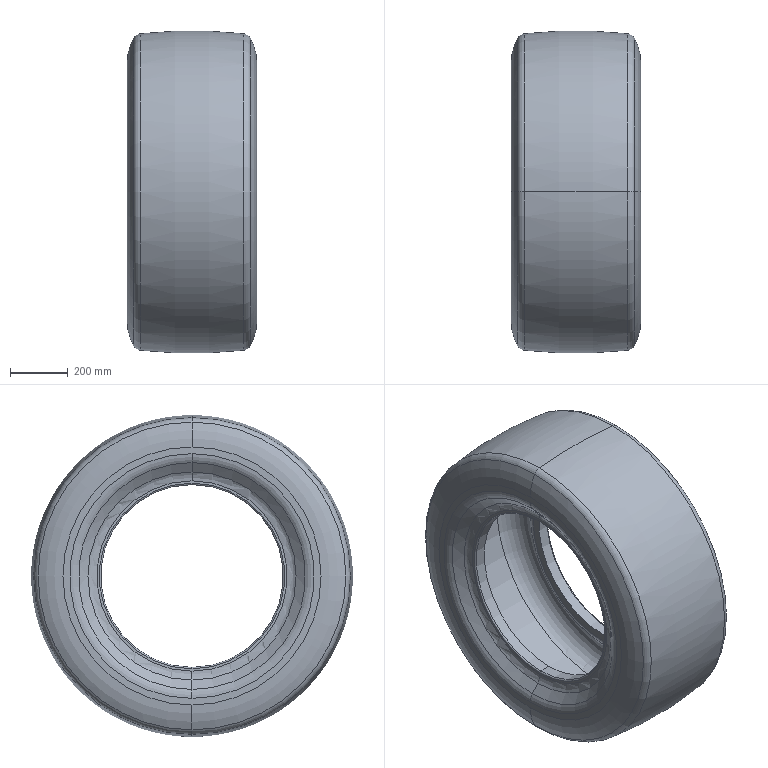Part | SolidWorks | features RevCut 1, Revolution 1 | 1 solid | 50 faces | box 450 x 1120 x 1120 mm | volume 112595756 mm3 | torus 30 | cone 8 | plane 6 | cylinder 6 | commonest cylinder face diameters 635 x4 1016 x2
STEP:
#1=CARTESIAN_POINT('',(142.639,0.,365.878));
#2=VERTEX_POINT('',#1);
#3=CARTESIAN_POINT('',(142.639,0.,-365.878));
#4=VERTEX_POINT('',#3);
#5=CARTESIAN_POINT('',(142.639,0.,0.));
#6=DIRECTION('',(-1.,0.,0.));
#7=DIRECTION('',(0.,0.,1.));
#8=AXIS2_PLACEMENT_3D('',#5,#6,#7);
#9=CIRCLE('',#8,365.878);
#10=EDGE_CURVE('',#2,#4,#9,.T.);
#11=ORIENTED_EDGE('',*,*,#10,.T.);
#12=CARTESIAN_POINT('',(134.,0.,-344.814));
#13=VERTEX_POINT('',#12);
#14=CARTESIAN_POINT('',(164.,0.,-344.814));
#15=DIRECTION('',(0.,1.,0.));
#16=DIRECTION('',(0.,0.,1.));
#17=AXIS2_PLACEMENT_3D('',#14,#15,#16);
#18=CIRCLE('',#17,30.);
#19=EDGE_CURVE('',#4,#13,#18,.T.);
#20=ORIENTED_EDGE('',*,*,#19,.T.);
#21=CARTESIAN_POINT('',(134.,0.,344.814));
#22=VERTEX_POINT('',#21);
#23=CARTESIAN_POINT('',(134.,0.,0.));
#24=DIRECTION('',(-1.,0.,0.));
#25=DIRECTION('',(0.,0.,1.));
#26=AXIS2_PLACEMENT_3D('',#23,#24,#25);
#27=CIRCLE('',#26,344.814);
#28=EDGE_CURVE('',#22,#13,#27,.T.);
#29=ORIENTED_EDGE('',*,*,#28,.F.);
#30=CARTESIAN_POINT('',(164.,0.,344.814));
#31=DIRECTION('',(0.,-1.,0.));
#32=DIRECTION('',(0.,0.,-1.));
#33=AXIS2_PLACEMENT_3D('',#30,#31,#32);
#34=CIRCLE('',#33,30.);
#35=EDGE_CURVE('',#2,#22,#34,.T.);
#36=ORIENTED_EDGE('',*,*,#35,.F.);
#37=EDGE_LOOP('',(#11,#20,#29,#36));
#38=FACE_OUTER_BOUND('',#37,.T.);
#39=CARTESIAN_POINT('',(164.,0.,0.));
#40=DIRECTION('',(-1.,0.,0.));
#41=DIRECTION('',(0.,0.,1.));
#42=AXIS2_PLACEMENT_3D('',#39,#40,#41);
#43=TOROIDAL_SURFACE('',#42,344.814,30.);
#44=ADVANCED_FACE('',(#38),#43,.T.);
#45=ORIENTED_EDGE('',*,*,#10,.F.);
#46=CARTESIAN_POINT('',(165.292,0.,388.849));
#47=VERTEX_POINT('',#46);
#48=CARTESIAN_POINT('',(165.292,0.,388.849));
#49=DIRECTION('',(0.7022,0.,0.712));
#50=VECTOR('',#49,1000.);
#51=LINE('',#48,#50);
#52=EDGE_CURVE('',#2,#47,#51,.T.);
#53=ORIENTED_EDGE('',*,*,#52,.T.);
#54=CARTESIAN_POINT('',(165.292,0.,-388.849));
#55=VERTEX_POINT('',#54);
#56=CARTESIAN_POINT('',(165.292,0.,0.));
#57=DIRECTION('',(-1.,0.,0.));
#58=DIRECTION('',(0.,0.,1.));
#59=AXIS2_PLACEMENT_3D('',#56,#57,#58);
#60=CIRCLE('',#59,388.849);
#61=EDGE_CURVE('',#47,#55,#60,.T.);
#62=ORIENTED_EDGE('',*,*,#61,.T.);
#63=CARTESIAN_POINT('',(165.292,0.,-388.849));
#64=DIRECTION('',(0.7022,0.,-0.712));
#65=VECTOR('',#64,1000.);
#66=LINE('',#63,#65);
#67=EDGE_CURVE('',#4,#55,#66,.T.);
#68=ORIENTED_EDGE('',*,*,#67,.F.);
#69=EDGE_LOOP('',(#45,#53,#62,#68));
#70=FACE_OUTER_BOUND('',#69,.T.);
#71=CARTESIAN_POINT('',(165.292,0.,0.));
#72=DIRECTION('',(1.,0.,0.));
#73=DIRECTION('',(0.,0.,-1.));
#74=AXIS2_PLACEMENT_3D('',#71,#72,#73);
#75=CONICAL_SURFACE('',#74,388.849,0.7924);
#76=ADVANCED_FACE('',(#70),#75,.T.);
#77=CARTESIAN_POINT('',(165.292,0.,0.));
#78=DIRECTION('',(-1.,0.,0.));
#79=DIRECTION('',(0.,0.,1.));
#80=AXIS2_PLACEMENT_3D('',#77,#78,#79);
#81=CIRCLE('',#80,388.849);
#82=EDGE_CURVE('',#55,#47,#81,.T.);
#83=ORIENTED_EDGE('',*,*,#82,.F.);
#84=CARTESIAN_POINT('',(115.45,0.,-508.));
#85=VERTEX_POINT('',#84);
#86=CARTESIAN_POINT('',(115.45,0.,-438.));
#87=DIRECTION('',(0.,1.,0.));
#88=DIRECTION('',(0.,0.,1.));
#89=AXIS2_PLACEMENT_3D('',#86,#87,#88);
#90=CIRCLE('',#89,70.);
#91=EDGE_CURVE('',#55,#85,#90,.T.);
#92=ORIENTED_EDGE('',*,*,#91,.T.);
#93=CARTESIAN_POINT('',(115.45,0.,508.));
#94=VERTEX_POINT('',#93);
#95=CARTESIAN_POINT('',(115.45,0.,0.));
#96=DIRECTION('',(-1.,0.,0.));
#97=DIRECTION('',(0.,0.,1.));
#98=AXIS2_PLACEMENT_3D('',#95,#96,#97);
#99=CIRCLE('',#98,508.);
#100=EDGE_CURVE('',#85,#94,#99,.T.);
#101=ORIENTED_EDGE('',*,*,#100,.T.);
#102=CARTESIAN_POINT('',(115.45,0.,438.));
#103=DIRECTION('',(0.,-1.,0.));
#104=DIRECTION('',(0.,0.,-1.));
#105=AXIS2_PLACEMENT_3D('',#102,#103,#104);
#106=CIRCLE('',#105,70.);
#107=EDGE_CURVE('',#47,#94,#106,.T.);
#108=ORIENTED_EDGE('',*,*,#107,.F.);
#109=EDGE_LOOP('',(#83,#92,#101,#108));
#110=FACE_OUTER_BOUND('',#109,.T.);
#111=CARTESIAN_POINT('',(115.45,0.,0.));
#112=DIRECTION('',(-1.,0.,0.));
#113=DIRECTION('',(0.,0.,1.));
#114=AXIS2_PLACEMENT_3D('',#111,#112,#113);
#115=TOROIDAL_SURFACE('',#114,438.,70.);
#116=ADVANCED_FACE('',(#110),#115,.F.);
#117=ORIENTED_EDGE('',*,*,#100,.F.);
#118=CARTESIAN_POINT('',(-115.45,0.,-508.));
#119=VERTEX_POINT('',#118);
#120=CARTESIAN_POINT('',(0.,0.,-508.));
#121=DIRECTION('',(-1.,0.,0.));
#122=VECTOR('',#121,1000.);
#123=LINE('',#120,#122);
#124=EDGE_CURVE('',#85,#119,#123,.T.);
#125=ORIENTED_EDGE('',*,*,#124,.T.);
#126=CARTESIAN_POINT('',(-115.45,0.,508.));
#127=VERTEX_POINT('',#126);
#128=CARTESIAN_POINT('',(-115.45,0.,0.));
#129=DIRECTION('',(-1.,0.,0.));
#130=DIRECTION('',(0.,0.,1.));
#131=AXIS2_PLACEMENT_3D('',#128,#129,#130);
#132=CIRCLE('',#131,508.);
#133=EDGE_CURVE('',#119,#127,#132,.T.);
#134=ORIENTED_EDGE('',*,*,#133,.T.);
#135=CARTESIAN_POINT('',(0.,0.,508.));
#136=DIRECTION('',(-1.,0.,0.));
#137=VECTOR('',#136,1000.);
#138=LINE('',#135,#137);
#139=EDGE_CURVE('',#94,#127,#138,.T.);
#140=ORIENTED_EDGE('',*,*,#139,.F.);
#141=EDGE_LOOP('',(#117,#125,#134,#140));
#142=FACE_OUTER_BOUND('',#141,.T.);
#143=CARTESIAN_POINT('',(0.,0.,0.));
#144=DIRECTION('',(-1.,0.,0.));
#145=DIRECTION('',(0.,0.,1.));
#146=AXIS2_PLACEMENT_3D('',#143,#144,#145);
#147=CYLINDRICAL_SURFACE('',#146,508.);
#148=ADVANCED_FACE('',(#142),#147,.F.);
#149=ORIENTED_EDGE('',*,*,#133,.F.);
#150=CARTESIAN_POINT('',(-165.292,0.,-388.849));
#151=VERTEX_POINT('',#150);
#152=CARTESIAN_POINT('',(-115.45,0.,-438.));
#153=DIRECTION('',(0.,1.,0.));
#154=DIRECTION('',(0.,0.,1.));
#155=AXIS2_PLACEMENT_3D('',#152,#153,#154);
#156=CIRCLE('',#155,70.);
#157=EDGE_CURVE('',#119,#151,#156,.T.);
#158=ORIENTED_EDGE('',*,*,#157,.T.);
#159=CARTESIAN_POINT('',(-165.292,0.,388.849));
#160=VERTEX_POINT('',#159);
#161=CARTESIAN_POINT('',(-165.292,0.,0.));
#162=DIRECTION('',(-1.,0.,0.));
#163=DIRECTION('',(0.,0.,1.));
#164=AXIS2_PLACEMENT_3D('',#161,#162,#163);
#165=CIRCLE('',#164,388.849);
#166=EDGE_CURVE('',#151,#160,#165,.T.);
#167=ORIENTED_EDGE('',*,*,#166,.T.);
#168=CARTESIAN_POINT('',(-115.45,0.,438.));
#169=DIRECTION('',(0.,-1.,0.));
#170=DIRECTION('',(0.,0.,-1.));
#171=AXIS2_PLACEMENT_3D('',#168,#169,#170);
#172=CIRCLE('',#171,70.);
#173=EDGE_CURVE('',#127,#160,#172,.T.);
#174=ORIENTED_EDGE('',*,*,#173,.F.);
#175=EDGE_LOOP('',(#149,#158,#167,#174));
#176=FACE_OUTER_BOUND('',#175,.T.);
#177=CARTESIAN_POINT('',(-115.45,0.,0.));
#178=DIRECTION('',(-1.,0.,0.));
#179=DIRECTION('',(0.,0.,1.));
#180=AXIS2_PLACEMENT_3D('',#177,#178,#179);
#181=TOROIDAL_SURFACE('',#180,438.,70.);
#182=ADVANCED_FACE('',(#176),#181,.F.);
#183=CARTESIAN_POINT('',(-142.639,0.,365.878));
#184=VERTEX_POINT('',#183);
#185=CARTESIAN_POINT('',(-142.639,0.,-365.878));
#186=VERTEX_POINT('',#185);
#187=CARTESIAN_POINT('',(-142.639,0.,0.));
#188=DIRECTION('',(-1.,0.,0.));
#189=DIRECTION('',(0.,0.,1.));
#190=AXIS2_PLACEMENT_3D('',#187,#188,#189);
#191=CIRCLE('',#190,365.878);
#192=EDGE_CURVE('',#184,#186,#191,.T.);
#193=ORIENTED_EDGE('',*,*,#192,.T.);
#194=CARTESIAN_POINT('',(-142.639,0.,-365.878));
#195=DIRECTION('',(-0.7022,0.,-0.712));
#196=VECTOR('',#195,1000.);
#197=LINE('',#194,#196);
#198=EDGE_CURVE('',#186,#151,#197,.T.);
#199=ORIENTED_EDGE('',*,*,#198,.T.);
#200=CARTESIAN_POINT('',(-165.292,0.,0.));
#201=DIRECTION('',(-1.,0.,0.));
#202=DIRECTION('',(0.,0.,1.));
#203=AXIS2_PLACEMENT_3D('',#200,#201,#202);
#204=CIRCLE('',#203,388.849);
#205=EDGE_CURVE('',#160,#151,#204,.T.);
#206=ORIENTED_EDGE('',*,*,#205,.F.);
#207=CARTESIAN_POINT('',(-142.639,0.,365.878));
#208=DIRECTION('',(-0.7022,0.,0.712));
#209=VECTOR('',#208,1000.);
#210=LINE('',#207,#209);
#211=EDGE_CURVE('',#184,#160,#210,.T.);
#212=ORIENTED_EDGE('',*,*,#211,.F.);
#213=EDGE_LOOP('',(#193,#199,#206,#212));
#214=FACE_OUTER_BOUND('',#213,.T.);
#215=CARTESIAN_POINT('',(-142.639,0.,0.));
#216=DIRECTION('',(-1.,0.,0.));
#217=DIRECTION('',(0.,0.,1.));
#218=AXIS2_PLACEMENT_3D('',#215,#216,#217);
#219=CONICAL_SURFACE('',#218,365.878,0.7924);
#220=ADVANCED_FACE('',(#214),#219,.T.);
#221=CARTESIAN_POINT('',(-134.,0.,344.814));
#222=VERTEX_POINT('',#221);
#223=CARTESIAN_POINT('',(-134.,0.,-344.814));
#224=VERTEX_POINT('',#223);
#225=CARTESIAN_POINT('',(-134.,0.,0.));
#226=DIRECTION('',(-1.,0.,0.));
#227=DIRECTION('',(0.,0.,1.));
#228=AXIS2_PLACEMENT_3D('',#225,#226,#227);
#229=CIRCLE('',#228,344.814);
#230=EDGE_CURVE('',#222,#224,#229,.T.);
#231=ORIENTED_EDGE('',*,*,#230,.T.);
#232=CARTESIAN_POINT('',(-164.,0.,-344.814));
#233=DIRECTION('',(0.,1.,0.));
#234=DIRECTION('',(0.,0.,1.));
#235=AXIS2_PLACEMENT_3D('',#232,#233,#234);
#236=CIRCLE('',#235,30.);
#237=EDGE_CURVE('',#224,#186,#236,.T.);
#238=ORIENTED_EDGE('',*,*,#237,.T.);
#239=ORIENTED_EDGE('',*,*,#192,.F.);
#240=CARTESIAN_POINT('',(-164.,0.,344.814));
#241=DIRECTION('',(0.,-1.,0.));
#242=DIRECTION('',(0.,0.,-1.));
#243=AXIS2_PLACEMENT_3D('',#240,#241,#242);
#244=CIRCLE('',#243,30.);
#245=EDGE_CURVE('',#222,#184,#244,.T.);
#246=ORIENTED_EDGE('',*,*,#245,.F.);
#247=EDGE_LOOP('',(#231,#238,#239,#246));
#248=FACE_OUTER_BOUND('',#247,.T.);
#249=CARTESIAN_POINT('',(-164.,0.,0.));
#250=DIRECTION('',(-1.,0.,0.));
#251=DIRECTION('',(0.,0.,1.));
#252=AXIS2_PLACEMENT_3D('',#249,#250,#251);
#253=TOROIDAL_SURFACE('',#252,344.814,30.);
#254=ADVANCED_FACE('',(#248),#253,.T.);
#255=CARTESIAN_POINT('',(173.,0.,-317.5));
#256=VERTEX_POINT('',#255);
#257=CARTESIAN_POINT('',(173.,0.,317.5));
#258=VERTEX_POINT('',#257);
#259=CARTESIAN_POINT('',(173.,0.,0.));
#260=DIRECTION('',(-1.,0.,0.));
#261=DIRECTION('',(0.,0.,1.));
#262=AXIS2_PLACEMENT_3D('',#259,#260,#261);
#263=CIRCLE('',#262,317.5);
#264=EDGE_CURVE('',#256,#258,#263,.T.);
#265=ORIENTED_EDGE('',*,*,#264,.F.);
#266=CARTESIAN_POINT('',(134.,0.,-317.5));
#267=VERTEX_POINT('',#266);
#268=CARTESIAN_POINT('',(0.,0.,-317.5));
#269=DIRECTION('',(-1.,0.,0.));
#270=VECTOR('',#269,1000.);
#271=LINE('',#268,#270);
#272=EDGE_CURVE('',#256,#267,#271,.T.);
#273=ORIENTED_EDGE('',*,*,#272,.T.);
#274=CARTESIAN_POINT('',(134.,0.,317.5));
#275=VERTEX_POINT('',#274);
#276=CARTESIAN_POINT('',(134.,0.,0.));
#277=DIRECTION('',(-1.,0.,0.));
#278=DIRECTION('',(0.,0.,1.));
#279=AXIS2_PLACEMENT_3D('',#276,#277,#278);
#280=CIRCLE('',#279,317.5);
#281=EDGE_CURVE('',#267,#275,#280,.T.);
#282=ORIENTED_EDGE('',*,*,#281,.T.);
#283=CARTESIAN_POINT('',(0.,0.,317.5));
#284=DIRECTION('',(-1.,0.,0.));
#285=VECTOR('',#284,1000.);
#286=LINE('',#283,#285);
#287=EDGE_CURVE('',#258,#275,#286,.T.);
#288=ORIENTED_EDGE('',*,*,#287,.F.);
#289=EDGE_LOOP('',(#265,#273,#282,#288));
#290=FACE_OUTER_BOUND('',#289,.T.);
#291=CARTESIAN_POINT('',(0.,0.,0.));
#292=DIRECTION('',(-1.,0.,0.));
#293=DIRECTION('',(0.,0.,1.));
#294=AXIS2_PLACEMENT_3D('',#291,#292,#293);
#295=CYLINDRICAL_SURFACE('',#294,317.5);
#296=ADVANCED_FACE('',(#290),#295,.F.);
#297=CARTESIAN_POINT('',(173.,0.,0.));
#298=DIRECTION('',(-1.,0.,0.));
#299=DIRECTION('',(0.,0.,1.));
#300=AXIS2_PLACEMENT_3D('',#297,#298,#299);
#301=CIRCLE('',#300,317.5);
#302=EDGE_CURVE('',#258,#256,#301,.T.);
#303=ORIENTED_EDGE('',*,*,#302,.T.);
#304=CARTESIAN_POINT('',(178.,0.,-322.5));
#305=VERTEX_POINT('',#304);
#306=CARTESIAN_POINT('',(173.,0.,-322.5));
#307=DIRECTION('',(0.,1.,0.));
#308=DIRECTION('',(0.,0.,1.));
#309=AXIS2_PLACEMENT_3D('',#306,#307,#308);
#310=CIRCLE('',#309,5.);
#311=EDGE_CURVE('',#256,#305,#310,.T.);
#312=ORIENTED_EDGE('',*,*,#311,.T.);
#313=CARTESIAN_POINT('',(178.,0.,322.5));
#314=VERTEX_POINT('',#313);
#315=CARTESIAN_POINT('',(178.,0.,0.));
#316=DIRECTION('',(-1.,0.,0.));
#317=DIRECTION('',(0.,0.,1.));
#318=AXIS2_PLACEMENT_3D('',#315,#316,#317);
#319=CIRCLE('',#318,322.5);
#320=EDGE_CURVE('',#314,#305,#319,.T.);
#321=ORIENTED_EDGE('',*,*,#320,.F.);
#322=CARTESIAN_POINT('',(173.,0.,322.5));
#323=DIRECTION('',(0.,-1.,0.));
#324=DIRECTION('',(0.,0.,-1.));
#325=AXIS2_PLACEMENT_3D('',#322,#323,#324);
#326=CIRCLE('',#325,5.);
#327=EDGE_CURVE('',#258,#314,#326,.T.);
#328=ORIENTED_EDGE('',*,*,#327,.F.);
#329=EDGE_LOOP('',(#303,#312,#321,#328));
#330=FACE_OUTER_BOUND('',#329,.T.);
#331=CARTESIAN_POINT('',(173.,0.,0.));
#332=DIRECTION('',(-1.,0.,0.));
#333=DIRECTION('',(0.,0.,1.));
#334=AXIS2_PLACEMENT_3D('',#331,#332,#333);
#335=TOROIDAL_SURFACE('',#334,322.5,5.);
#336=ADVANCED_FACE('',(#330),#335,.T.);
#337=CARTESIAN_POINT('',(188.653,0.,-361.58));
#338=VERTEX_POINT('',#337);
#339=CARTESIAN_POINT('',(188.653,0.,361.58));
#340=VERTEX_POINT('',#339);
#341=CARTESIAN_POINT('',(188.653,0.,0.));
#342=DIRECTION('',(-1.,0.,0.));
#343=DIRECTION('',(0.,0.,1.));
#344=AXIS2_PLACEMENT_3D('',#341,#342,#343);
#345=CIRCLE('',#344,361.58);
#346=EDGE_CURVE('',#338,#340,#345,.T.);
#347=ORIENTED_EDGE('',*,*,#346,.F.);
#348=CARTESIAN_POINT('',(178.,0.,-330.728));
#349=VERTEX_POINT('',#348);
#350=CARTESIAN_POINT('',(228.,0.,-330.728));
#351=DIRECTION('',(0.,1.,0.));
#352=DIRECTION('',(0.,0.,1.));
#353=AXIS2_PLACEMENT_3D('',#350,#351,#352);
#354=CIRCLE('',#353,50.);
#355=EDGE_CURVE('',#338,#349,#354,.T.);
#356=ORIENTED_EDGE('',*,*,#355,.T.);
#357=CARTESIAN_POINT('',(178.,0.,330.728));
#358=VERTEX_POINT('',#357);
#359=CARTESIAN_POINT('',(178.,0.,0.));
#360=DIRECTION('',(-1.,0.,0.));
#361=DIRECTION('',(0.,0.,1.));
#362=AXIS2_PLACEMENT_3D('',#359,#360,#361);
#363=CIRCLE('',#362,330.728);
#364=EDGE_CURVE('',#349,#358,#363,.T.);
#365=ORIENTED_EDGE('',*,*,#364,.T.);
#366=CARTESIAN_POINT('',(228.,0.,330.728));
#367=DIRECTION('',(0.,-1.,0.));
#368=DIRECTION('',(0.,0.,-1.));
#369=AXIS2_PLACEMENT_3D('',#366,#367,#368);
#370=CIRCLE('',#369,50.);
#371=EDGE_CURVE('',#340,#358,#370,.T.);
#372=ORIENTED_EDGE('',*,*,#371,.F.);
#373=EDGE_LOOP('',(#347,#356,#365,#372));
#374=FACE_OUTER_BOUND('',#373,.T.);
#375=CARTESIAN_POINT('',(228.,0.,0.));
#376=DIRECTION('',(-1.,0.,0.));
#377=DIRECTION('',(0.,0.,1.));
#378=AXIS2_PLACEMENT_3D('',#375,#376,#377);
#379=TOROIDAL_SURFACE('',#378,330.728,50.);
#380=ADVANCED_FACE('',(#374),#379,.F.);
#381=ORIENTED_EDGE('',*,*,#346,.T.);
#382=CARTESIAN_POINT('',(214.347,0.,394.348));
#383=VERTEX_POINT('',#382);
#384=CARTESIAN_POINT('',(188.653,0.,361.58));
#385=DIRECTION('',(0.617,0.,0.7869));
#386=VECTOR('',#385,1000.);
#387=LINE('',#384,#386);
#388=EDGE_CURVE('',#340,#383,#387,.T.);
#389=ORIENTED_EDGE('',*,*,#388,.T.);
#390=CARTESIAN_POINT('',(214.347,0.,-394.348));
#391=VERTEX_POINT('',#390);
#392=CARTESIAN_POINT('',(214.347,0.,0.));
#393=DIRECTION('',(-1.,0.,0.));
#394=DIRECTION('',(0.,0.,1.));
#395=AXIS2_PLACEMENT_3D('',#392,#393,#394);
#396=CIRCLE('',#395,394.348);
#397=EDGE_CURVE('',#391,#383,#396,.T.);
#398=ORIENTED_EDGE('',*,*,#397,.F.);
#399=CARTESIAN_POINT('',(188.653,0.,-361.58));
#400=DIRECTION('',(0.617,0.,-0.7869));
#401=VECTOR('',#400,1000.);
#402=LINE('',#399,#401);
#403=EDGE_CURVE('',#338,#391,#402,.T.);
#404=ORIENTED_EDGE('',*,*,#403,.F.);
#405=EDGE_LOOP('',(#381,#389,#398,#404));
#406=FACE_OUTER_BOUND('',#405,.T.);
#407=CARTESIAN_POINT('',(188.653,0.,0.));
#408=DIRECTION('',(1.,0.,0.));
#409=DIRECTION('',(0.,0.,-1.));
#410=AXIS2_PLACEMENT_3D('',#407,#408,#409);
#411=CONICAL_SURFACE('',#410,361.58,0.9058);
#412=ADVANCED_FACE('',(#406),#411,.F.);
#413=CARTESIAN_POINT('',(214.347,0.,0.));
#414=DIRECTION('',(-1.,0.,0.));
#415=DIRECTION('',(0.,0.,1.));
#416=AXIS2_PLACEMENT_3D('',#413,#414,#415);
#417=CIRCLE('',#416,394.348);
#418=EDGE_CURVE('',#383,#391,#417,.T.);
#419=ORIENTED_EDGE('',*,*,#418,.T.);
#420=CARTESIAN_POINT('',(225.,0.,-425.2));
#421=VERTEX_POINT('',#420);
#422=CARTESIAN_POINT('',(175.,0.,-425.2));
#423=DIRECTION('',(0.,1.,0.));
#424=DIRECTION('',(0.,0.,1.));
#425=AXIS2_PLACEMENT_3D('',#422,#423,#424);
#426=CIRCLE('',#425,50.);
#427=EDGE_CURVE('',#391,#421,#426,.T.);
#428=ORIENTED_EDGE('',*,*,#427,.T.);
#429=CARTESIAN_POINT('',(225.,0.,425.2));
#430=VERTEX_POINT('',#429);
#431=CARTESIAN_POINT('',(225.,0.,0.));
#432=DIRECTION('',(-1.,0.,0.));
#433=DIRECTION('',(0.,0.,1.));
#434=AXIS2_PLACEMENT_3D('',#431,#432,#433);
#435=CIRCLE('',#434,425.2);
#436=EDGE_CURVE('',#430,#421,#435,.T.);
#437=ORIENTED_EDGE('',*,*,#436,.F.);
#438=CARTESIAN_POINT('',(175.,0.,425.2));
#439=DIRECTION('',(0.,-1.,0.));
#440=DIRECTION('',(0.,0.,-1.));
#441=AXIS2_PLACEMENT_3D('',#438,#439,#440);
#442=CIRCLE('',#441,50.);
#443=EDGE_CURVE('',#383,#430,#442,.T.);
#444=ORIENTED_EDGE('',*,*,#443,.F.);
#445=EDGE_LOOP('',(#419,#428,#437,#444));
#446=FACE_OUTER_BOUND('',#445,.T.);
#447=CARTESIAN_POINT('',(175.,0.,0.));
#448=DIRECTION('',(-1.,0.,0.));
#449=DIRECTION('',(0.,0.,1.));
#450=AXIS2_PLACEMENT_3D('',#447,#448,#449);
#451=TOROIDAL_SURFACE('',#450,425.2,50.);
#452=ADVANCED_FACE('',(#446),#451,.T.);
#453=CARTESIAN_POINT('',(225.,0.,448.5));
#454=VERTEX_POINT('',#453);
#455=CARTESIAN_POINT('',(225.,0.,-448.5));
#456=VERTEX_POINT('',#455);
#457=CARTESIAN_POINT('',(225.,0.,0.));
#458=DIRECTION('',(-1.,0.,0.));
#459=DIRECTION('',(0.,0.,1.));
#460=AXIS2_PLACEMENT_3D('',#457,#458,#459);
#461=CIRCLE('',#460,448.5);
#462=EDGE_CURVE('',#454,#456,#461,.T.);
#463=ORIENTED_EDGE('',*,*,#462,.T.);
#464=CARTESIAN_POINT('',(203.093,0.,-534.562));
#465=VERTEX_POINT('',#464);
#466=CARTESIAN_POINT('',(45.,0.,-448.5));
#467=DIRECTION('',(0.,1.,0.));
#468=DIRECTION('',(0.,0.,1.));
#469=AXIS2_PLACEMENT_3D('',#466,#467,#468);
#470=CIRCLE('',#469,180.);
#471=EDGE_CURVE('',#456,#465,#470,.T.);
#472=ORIENTED_EDGE('',*,*,#471,.T.);
#473=CARTESIAN_POINT('',(203.093,0.,534.562));
#474=VERTEX_POINT('',#473);
#475=CARTESIAN_POINT('',(203.093,0.,0.));
#476=DIRECTION('',(-1.,0.,0.));
#477=DIRECTION('',(0.,0.,1.));
#478=AXIS2_PLACEMENT_3D('',#475,#476,#477);
#479=CIRCLE('',#478,534.562);
#480=EDGE_CURVE('',#474,#465,#479,.T.);
#481=ORIENTED_EDGE('',*,*,#480,.F.);
#482=CARTESIAN_POINT('',(45.,0.,448.5));
#483=DIRECTION('',(0.,-1.,0.));
#484=DIRECTION('',(0.,0.,-1.));
#485=AXIS2_PLACEMENT_3D('',#482,#483,#484);
#486=CIRCLE('',#485,180.);
#487=EDGE_CURVE('',#454,#474,#486,.T.);
#488=ORIENTED_EDGE('',*,*,#487,.F.);
#489=EDGE_LOOP('',(#463,#472,#481,#488));
#490=FACE_OUTER_BOUND('',#489,.T.);
#491=CARTESIAN_POINT('',(45.,0.,0.));
#492=DIRECTION('',(-1.,0.,0.));
#493=DIRECTION('',(0.,0.,1.));
#494=AXIS2_PLACEMENT_3D('',#491,#492,#493);
#495=TOROIDAL_SURFACE('',#494,448.5,180.);
#496=ADVANCED_FACE('',(#490),#495,.T.);
#497=ORIENTED_EDGE('',*,*,#480,.T.);
#498=CARTESIAN_POINT('',(180.054,0.,-550.035));
#499=VERTEX_POINT('',#498);
#500=CARTESIAN_POINT('',(176.744,0.,-520.218));
#501=DIRECTION('',(0.,1.,0.));
#502=DIRECTION('',(0.,0.,1.));
#503=AXIS2_PLACEMENT_3D('',#500,#501,#502);
#504=CIRCLE('',#503,30.);
#505=EDGE_CURVE('',#465,#499,#504,.T.);
#506=ORIENTED_EDGE('',*,*,#505,.T.);
#507=CARTESIAN_POINT('',(180.054,0.,550.035));
#508=VERTEX_POINT('',#507);
#509=CARTESIAN_POINT('',(180.054,0.,0.));
#510=DIRECTION('',(-1.,0.,0.));
#511=DIRECTION('',(0.,0.,1.));
#512=AXIS2_PLACEMENT_3D('',#509,#510,#511);
#513=CIRCLE('',#512,550.035);
#514=EDGE_CURVE('',#508,#499,#513,.T.);
#515=ORIENTED_EDGE('',*,*,#514,.F.);
#516=CARTESIAN_POINT('',(176.744,0.,520.218));
#517=DIRECTION('',(0.,-1.,0.));
#518=DIRECTION('',(0.,0.,-1.));
#519=AXIS2_PLACEMENT_3D('',#516,#517,#518);
#520=CIRCLE('',#519,30.);
#521=EDGE_CURVE('',#474,#508,#520,.T.);
#522=ORIENTED_EDGE('',*,*,#521,.F.);
#523=EDGE_LOOP('',(#497,#506,#515,#522));
#524=FACE_OUTER_BOUND('',#523,.T.);
#525=CARTESIAN_POINT('',(176.744,0.,0.));
#526=DIRECTION('',(-1.,0.,0.));
#527=DIRECTION('',(0.,0.,1.));
#528=AXIS2_PLACEMENT_3D('',#525,#526,#527);
#529=TOROIDAL_SURFACE('',#528,520.218,30.);
#530=ADVANCED_FACE('',(#524),#529,.T.);
#531=ORIENTED_EDGE('',*,*,#514,.T.);
#532=CARTESIAN_POINT('',(-180.054,0.,-550.035));
#533=VERTEX_POINT('',#532);
#534=CARTESIAN_POINT('',(0.,0.,1071.7));
#535=DIRECTION('',(0.,1.,0.));
#536=DIRECTION('',(0.,0.,1.));
#537=AXIS2_PLACEMENT_3D('',#534,#535,#536);
#538=CIRCLE('',#537,1631.7);
#539=EDGE_CURVE('',#499,#533,#538,.T.);
#540=ORIENTED_EDGE('',*,*,#539,.T.);
#541=CARTESIAN_POINT('',(-180.054,0.,550.035));
#542=VERTEX_POINT('',#541);
#543=CARTESIAN_POINT('',(-180.054,0.,0.));
#544=DIRECTION('',(-1.,0.,0.));
#545=DIRECTION('',(0.,0.,1.));
#546=AXIS2_PLACEMENT_3D('',#543,#544,#545);
#547=CIRCLE('',#546,550.035);
#548=EDGE_CURVE('',#542,#533,#547,.T.);
#549=ORIENTED_EDGE('',*,*,#548,.F.);
#550=CARTESIAN_POINT('',(0.,0.,-1071.7));
#551=DIRECTION('',(0.,-1.,0.));
#552=DIRECTION('',(0.,0.,-1.));
#553=AXIS2_PLACEMENT_3D('',#550,#551,#552);
#554=CIRCLE('',#553,1631.7);
#555=EDGE_CURVE('',#508,#542,#554,.T.);
#556=ORIENTED_EDGE('',*,*,#555,.F.);
#557=EDGE_LOOP('',(#531,#540,#549,#556));
#558=FACE_OUTER_BOUND('',#557,.T.);
#559=CARTESIAN_POINT('',(0.,0.,0.));
#560=DIRECTION('',(-1.,0.,0.));
#561=DIRECTION('',(0.,0.,1.));
#562=AXIS2_PLACEMENT_3D('',#559,#560,#561);
#563=TOROIDAL_SURFACE('',#562,-1071.7,1631.7);
#564=ADVANCED_FACE('',(#558),#563,.T.);
#565=ORIENTED_EDGE('',*,*,#548,.T.);
#566=CARTESIAN_POINT('',(-203.093,0.,-534.562));
#567=VERTEX_POINT('',#566);
#568=CARTESIAN_POINT('',(-176.744,0.,-520.218));
#569=DIRECTION('',(0.,1.,0.));
#570=DIRECTION('',(0.,0.,1.));
#571=AXIS2_PLACEMENT_3D('',#568,#569,#570);
#572=CIRCLE('',#571,30.);
#573=EDGE_CURVE('',#533,#567,#572,.T.);
#574=ORIENTED_EDGE('',*,*,#573,.T.);
#575=CARTESIAN_POINT('',(-203.093,0.,534.562));
#576=VERTEX_POINT('',#575);
#577=CARTESIAN_POINT('',(-203.093,0.,0.));
#578=DIRECTION('',(-1.,0.,0.));
#579=DIRECTION('',(0.,0.,1.));
#580=AXIS2_PLACEMENT_3D('',#577,#578,#579);
#581=CIRCLE('',#580,534.562);
#582=EDGE_CURVE('',#576,#567,#581,.T.);
#583=ORIENTED_EDGE('',*,*,#582,.F.);
#584=CARTESIAN_POINT('',(-176.744,0.,520.218));
#585=DIRECTION('',(0.,-1.,0.));
#586=DIRECTION('',(0.,0.,-1.));
#587=AXIS2_PLACEMENT_3D('',#584,#585,#586);
#588=CIRCLE('',#587,30.);
#589=EDGE_CURVE('',#542,#576,#588,.T.);
#590=ORIENTED_EDGE('',*,*,#589,.F.);
#591=EDGE_LOOP('',(#565,#574,#583,#590));
#592=FACE_OUTER_BOUND('',#591,.T.);
#593=CARTESIAN_POINT('',(-176.744,0.,0.));
#594=DIRECTION('',(-1.,0.,0.));
#595=DIRECTION('',(0.,0.,1.));
#596=AXIS2_PLACEMENT_3D('',#593,#594,#595);
#597=TOROIDAL_SURFACE('',#596,520.218,30.);
#598=ADVANCED_FACE('',(#592),#597,.T.);
#599=ORIENTED_EDGE('',*,*,#582,.T.);
#600=CARTESIAN_POINT('',(-225.,0.,-448.5));
#601=VERTEX_POINT('',#600);
#602=CARTESIAN_POINT('',(-45.,0.,-448.5));
#603=DIRECTION('',(0.,1.,0.));
#604=DIRECTION('',(0.,0.,1.));
#605=AXIS2_PLACEMENT_3D('',#602,#603,#604);
#606=CIRCLE('',#605,180.);
#607=EDGE_CURVE('',#567,#601,#606,.T.);
#608=ORIENTED_EDGE('',*,*,#607,.T.);
#609=CARTESIAN_POINT('',(-225.,0.,448.5));
#610=VERTEX_POINT('',#609);
#611=CARTESIAN_POINT('',(-225.,0.,0.));
#612=DIRECTION('',(-1.,0.,0.));
#613=DIRECTION('',(0.,0.,1.));
#614=AXIS2_PLACEMENT_3D('',#611,#612,#613);
#615=CIRCLE('',#614,448.5);
#616=EDGE_CURVE('',#610,#601,#615,.T.);
#617=ORIENTED_EDGE('',*,*,#616,.F.);
#618=CARTESIAN_POINT('',(-45.,0.,448.5));
#619=DIRECTION('',(0.,-1.,0.));
#620=DIRECTION('',(0.,0.,-1.));
#621=AXIS2_PLACEMENT_3D('',#618,#619,#620);
#622=CIRCLE('',#621,180.);
#623=EDGE_CURVE('',#576,#610,#622,.T.);
#624=ORIENTED_EDGE('',*,*,#623,.F.);
#625=EDGE_LOOP('',(#599,#608,#617,#624));
#626=FACE_OUTER_BOUND('',#625,.T.);
#627=CARTESIAN_POINT('',(-45.,0.,0.));
#628=DIRECTION('',(-1.,0.,0.));
#629=DIRECTION('',(0.,0.,1.));
#630=AXIS2_PLACEMENT_3D('',#627,#628,#629);
#631=TOROIDAL_SURFACE('',#630,448.5,180.);
#632=ADVANCED_FACE('',(#626),#631,.T.);
#633=CARTESIAN_POINT('',(-225.,0.,425.2));
#634=VERTEX_POINT('',#633);
#635=CARTESIAN_POINT('',(-225.,0.,-425.2));
#636=VERTEX_POINT('',#635);
#637=CARTESIAN_POINT('',(-225.,0.,0.));
#638=DIRECTION('',(-1.,0.,0.));
#639=DIRECTION('',(0.,0.,1.));
#640=AXIS2_PLACEMENT_3D('',#637,#638,#639);
#641=CIRCLE('',#640,425.2);
#642=EDGE_CURVE('',#634,#636,#641,.T.);
#643=ORIENTED_EDGE('',*,*,#642,.T.);
#644=CARTESIAN_POINT('',(-214.347,0.,-394.348));
#645=VERTEX_POINT('',#644);
#646=CARTESIAN_POINT('',(-175.,0.,-425.2));
#647=DIRECTION('',(0.,1.,0.));
#648=DIRECTION('',(0.,0.,1.));
#649=AXIS2_PLACEMENT_3D('',#646,#647,#648);
#650=CIRCLE('',#649,50.);
#651=EDGE_CURVE('',#636,#645,#650,.T.);
#652=ORIENTED_EDGE('',*,*,#651,.T.);
#653=CARTESIAN_POINT('',(-214.347,0.,394.348));
#654=VERTEX_POINT('',#653);
#655=CARTESIAN_POINT('',(-214.347,0.,0.));
#656=DIRECTION('',(-1.,0.,0.));
#657=DIRECTION('',(0.,0.,1.));
#658=AXIS2_PLACEMENT_3D('',#655,#656,#657);
#659=CIRCLE('',#658,394.348);
#660=EDGE_CURVE('',#654,#645,#659,.T.);
#661=ORIENTED_EDGE('',*,*,#660,.F.);
#662=CARTESIAN_POINT('',(-175.,0.,425.2));
#663=DIRECTION('',(0.,-1.,0.));
#664=DIRECTION('',(0.,0.,-1.));
#665=AXIS2_PLACEMENT_3D('',#662,#663,#664);
#666=CIRCLE('',#665,50.);
#667=EDGE_CURVE('',#634,#654,#666,.T.);
#668=ORIENTED_EDGE('',*,*,#667,.F.);
#669=EDGE_LOOP('',(#643,#652,#661,#668));
#670=FACE_OUTER_BOUND('',#669,.T.);
#671=CARTESIAN_POINT('',(-175.,0.,0.));
#672=DIRECTION('',(-1.,0.,0.));
#673=DIRECTION('',(0.,0.,1.));
#674=AXIS2_PLACEMENT_3D('',#671,#672,#673);
#675=TOROIDAL_SURFACE('',#674,425.2,50.);
#676=ADVANCED_FACE('',(#670),#675,.T.);
#677=CARTESIAN_POINT('',(-188.653,0.,-361.58));
#678=VERTEX_POINT('',#677);
#679=CARTESIAN_POINT('',(-188.653,0.,361.58));
#680=VERTEX_POINT('',#679);
#681=CARTESIAN_POINT('',(-188.653,0.,0.));
#682=DIRECTION('',(-1.,0.,0.));
#683=DIRECTION('',(0.,0.,1.));
#684=AXIS2_PLACEMENT_3D('',#681,#682,#683);
#685=CIRCLE('',#684,361.58);
#686=EDGE_CURVE('',#678,#680,#685,.T.);
#687=ORIENTED_EDGE('',*,*,#686,.F.);
#688=CARTESIAN_POINT('',(-214.347,0.,-394.348));
#689=DIRECTION('',(-0.617,0.,-0.7869));
#690=VECTOR('',#689,1000.);
#691=LINE('',#688,#690);
#692=EDGE_CURVE('',#678,#645,#691,.T.);
#693=ORIENTED_EDGE('',*,*,#692,.T.);
#694=CARTESIAN_POINT('',(-214.347,0.,0.));
#695=DIRECTION('',(-1.,0.,0.));
#696=DIRECTION('',(0.,0.,1.));
#697=AXIS2_PLACEMENT_3D('',#694,#695,#696);
#698=CIRCLE('',#697,394.348);
#699=EDGE_CURVE('',#645,#654,#698,.T.);
#700=ORIENTED_EDGE('',*,*,#699,.T.);
#701=CARTESIAN_POINT('',(-214.347,0.,394.348));
#702=DIRECTION('',(-0.617,0.,0.7869));
#703=VECTOR('',#702,1000.);
#704=LINE('',#701,#703);
#705=EDGE_CURVE('',#680,#654,#704,.T.);
#706=ORIENTED_EDGE('',*,*,#705,.F.);
#707=EDGE_LOOP('',(#687,#693,#700,#706));
#708=FACE_OUTER_BOUND('',#707,.T.);
#709=CARTESIAN_POINT('',(-214.347,0.,0.));
#710=DIRECTION('',(-1.,0.,0.));
#711=DIRECTION('',(0.,0.,1.));
#712=AXIS2_PLACEMENT_3D('',#709,#710,#711);
#713=CONICAL_SURFACE('',#712,394.348,0.9058);
#714=ADVANCED_FACE('',(#708),#713,.F.);
#715=CARTESIAN_POINT('',(-178.,0.,-330.728));
#716=VERTEX_POINT('',#715);
#717=CARTESIAN_POINT('',(-178.,0.,330.728));
#718=VERTEX_POINT('',#717);
#719=CARTESIAN_POINT('',(-178.,0.,0.));
#720=DIRECTION('',(-1.,0.,0.));
#721=DIRECTION('',(0.,0.,1.));
#722=AXIS2_PLACEMENT_3D('',#719,#720,#721);
#723=CIRCLE('',#722,330.728);
#724=EDGE_CURVE('',#716,#718,#723,.T.);
#725=ORIENTED_EDGE('',*,*,#724,.F.);
#726=CARTESIAN_POINT('',(-228.,0.,-330.728));
#727=DIRECTION('',(0.,1.,0.));
#728=DIRECTION('',(0.,0.,1.));
#729=AXIS2_PLACEMENT_3D('',#726,#727,#728);
#730=CIRCLE('',#729,50.);
#731=EDGE_CURVE('',#716,#678,#730,.T.);
#732=ORIENTED_EDGE('',*,*,#731,.T.);
#733=ORIENTED_EDGE('',*,*,#686,.T.);
#734=CARTESIAN_POINT('',(-228.,0.,330.728));
#735=DIRECTION('',(0.,-1.,0.));
#736=DIRECTION('',(0.,0.,-1.));
#737=AXIS2_PLACEMENT_3D('',#734,#735,#736);
#738=CIRCLE('',#737,50.);
#739=EDGE_CURVE('',#718,#680,#738,.T.);
#740=ORIENTED_EDGE('',*,*,#739,.F.);
#741=EDGE_LOOP('',(#725,#732,#733,#740));
#742=FACE_OUTER_BOUND('',#741,.T.);
#743=CARTESIAN_POINT('',(-228.,0.,0.));
#744=DIRECTION('',(-1.,0.,0.));
#745=DIRECTION('',(0.,0.,1.));
#746=AXIS2_PLACEMENT_3D('',#743,#744,#745);
#747=TOROIDAL_SURFACE('',#746,330.728,50.);
#748=ADVANCED_FACE('',(#742),#747,.F.);
#749=CARTESIAN_POINT('',(-178.,0.,322.5));
#750=VERTEX_POINT('',#749);
#751=CARTESIAN_POINT('',(-178.,0.,-322.5));
#752=VERTEX_POINT('',#751);
#753=CARTESIAN_POINT('',(-178.,0.,0.));
#754=DIRECTION('',(-1.,0.,0.));
#755=DIRECTION('',(0.,0.,1.));
#756=AXIS2_PLACEMENT_3D('',#753,#754,#755);
#757=CIRCLE('',#756,322.5);
#758=EDGE_CURVE('',#750,#752,#757,.T.);
#759=ORIENTED_EDGE('',*,*,#758,.T.);
#760=CARTESIAN_POINT('',(-173.,0.,-317.5));
#761=VERTEX_POINT('',#760);
#762=CARTESIAN_POINT('',(-173.,0.,-322.5));
#763=DIRECTION('',(0.,1.,0.));
#764=DIRECTION('',(0.,0.,1.));
#765=AXIS2_PLACEMENT_3D('',#762,#763,#764);
#766=CIRCLE('',#765,5.);
#767=EDGE_CURVE('',#752,#761,#766,.T.);
#768=ORIENTED_EDGE('',*,*,#767,.T.);
#769=CARTESIAN_POINT('',(-173.,0.,317.5));
#770=VERTEX_POINT('',#769);
#771=CARTESIAN_POINT('',(-173.,0.,0.));
#772=DIRECTION('',(-1.,0.,0.));
#773=DIRECTION('',(0.,0.,1.));
#774=AXIS2_PLACEMENT_3D('',#771,#772,#773);
#775=CIRCLE('',#774,317.5);
#776=EDGE_CURVE('',#770,#761,#775,.T.);
#777=ORIENTED_EDGE('',*,*,#776,.F.);
#778=CARTESIAN_POINT('',(-173.,0.,322.5));
#779=DIRECTION('',(0.,-1.,0.));
#780=DIRECTION('',(0.,0.,-1.));
#781=AXIS2_PLACEMENT_3D('',#778,#779,#780);
#782=CIRCLE('',#781,5.);
#783=EDGE_CURVE('',#750,#770,#782,.T.);
#784=ORIENTED_EDGE('',*,*,#783,.F.);
#785=EDGE_LOOP('',(#759,#768,#777,#784));
#786=FACE_OUTER_BOUND('',#785,.T.);
#787=CARTESIAN_POINT('',(-173.,0.,0.));
#788=DIRECTION('',(-1.,0.,0.));
#789=DIRECTION('',(0.,0.,1.));
#790=AXIS2_PLACEMENT_3D('',#787,#788,#789);
#791=TOROIDAL_SURFACE('',#790,322.5,5.);
#792=ADVANCED_FACE('',(#786),#791,.T.);
#793=CARTESIAN_POINT('',(-134.,0.,-317.5));
#794=VERTEX_POINT('',#793);
#795=CARTESIAN_POINT('',(-134.,0.,317.5));
#796=VERTEX_POINT('',#795);
#797=CARTESIAN_POINT('',(-134.,0.,0.));
#798=DIRECTION('',(-1.,0.,0.));
#799=DIRECTION('',(0.,0.,1.));
#800=AXIS2_PLACEMENT_3D('',#797,#798,#799);
#801=CIRCLE('',#800,317.5);
#802=EDGE_CURVE('',#794,#796,#801,.T.);
#803=ORIENTED_EDGE('',*,*,#802,.F.);
#804=CARTESIAN_POINT('',(0.,0.,-317.5));
#805=DIRECTION('',(-1.,0.,0.));
#806=VECTOR('',#805,1000.);
#807=LINE('',#804,#806);
#808=EDGE_CURVE('',#794,#761,#807,.T.);
#809=ORIENTED_EDGE('',*,*,#808,.T.);
#810=CARTESIAN_POINT('',(-173.,0.,0.));
#811=DIRECTION('',(-1.,0.,0.));
#812=DIRECTION('',(0.,0.,1.));
#813=AXIS2_PLACEMENT_3D('',#810,#811,#812);
#814=CIRCLE('',#813,317.5);
#815=EDGE_CURVE('',#761,#770,#814,.T.);
#816=ORIENTED_EDGE('',*,*,#815,.T.);
#817=CARTESIAN_POINT('',(0.,0.,317.5));
#818=DIRECTION('',(-1.,0.,0.));
#819=VECTOR('',#818,1000.);
#820=LINE('',#817,#819);
#821=EDGE_CURVE('',#796,#770,#820,.T.);
#822=ORIENTED_EDGE('',*,*,#821,.F.);
#823=EDGE_LOOP('',(#803,#809,#816,#822));
#824=FACE_OUTER_BOUND('',#823,.T.);
#825=CARTESIAN_POINT('',(0.,0.,0.));
#826=DIRECTION('',(-1.,0.,0.));
#827=DIRECTION('',(0.,0.,1.));
#828=AXIS2_PLACEMENT_3D('',#825,#826,#827);
#829=CYLINDRICAL_SURFACE('',#828,317.5);
#830=ADVANCED_FACE('',(#824),#829,.F.);
#831=ORIENTED_EDGE('',*,*,#808,.F.);
#832=CARTESIAN_POINT('',(-134.,0.,0.));
#833=DIRECTION('',(-1.,0.,0.));
#834=DIRECTION('',(0.,0.,1.));
#835=AXIS2_PLACEMENT_3D('',#832,#833,#834);
#836=CIRCLE('',#835,317.5);
#837=EDGE_CURVE('',#796,#794,#836,.T.);
#838=ORIENTED_EDGE('',*,*,#837,.F.);
#839=ORIENTED_EDGE('',*,*,#821,.T.);
#840=ORIENTED_EDGE('',*,*,#776,.T.);
#841=EDGE_LOOP('',(#831,#838,#839,#840));
#842=FACE_OUTER_BOUND('',#841,.T.);
#843=CARTESIAN_POINT('',(0.,0.,0.));
#844=DIRECTION('',(-1.,0.,0.));
#845=DIRECTION('',(0.,0.,1.));
#846=AXIS2_PLACEMENT_3D('',#843,#844,#845);
#847=CYLINDRICAL_SURFACE('',#846,317.5);
#848=ADVANCED_FACE('',(#842),#847,.F.);
#849=ORIENTED_EDGE('',*,*,#767,.F.);
#850=CARTESIAN_POINT('',(-178.,0.,0.));
#851=DIRECTION('',(-1.,0.,0.));
#852=DIRECTION('',(0.,0.,1.));
#853=AXIS2_PLACEMENT_3D('',#850,#851,#852);
#854=CIRCLE('',#853,322.5);
#855=EDGE_CURVE('',#752,#750,#854,.T.);
#856=ORIENTED_EDGE('',*,*,#855,.T.);
#857=ORIENTED_EDGE('',*,*,#783,.T.);
#858=ORIENTED_EDGE('',*,*,#815,.F.);
#859=EDGE_LOOP('',(#849,#856,#857,#858));
#860=FACE_OUTER_BOUND('',#859,.T.);
#861=CARTESIAN_POINT('',(-173.,0.,0.));
#862=DIRECTION('',(-1.,0.,0.));
#863=DIRECTION('',(0.,0.,1.));
#864=AXIS2_PLACEMENT_3D('',#861,#862,#863);
#865=TOROIDAL_SURFACE('',#864,322.5,5.);
#866=ADVANCED_FACE('',(#860),#865,.T.);
#867=ORIENTED_EDGE('',*,*,#758,.F.);
#868=ORIENTED_EDGE('',*,*,#855,.F.);
#869=EDGE_LOOP('',(#867,#868));
#870=FACE_BOUND('',#869,.T.);
#871=CARTESIAN_POINT('',(-178.,0.,0.));
#872=DIRECTION('',(-1.,0.,0.));
#873=DIRECTION('',(0.,0.,1.));
#874=AXIS2_PLACEMENT_3D('',#871,#872,#873);
#875=CIRCLE('',#874,330.728);
#876=EDGE_CURVE('',#718,#716,#875,.T.);
#877=ORIENTED_EDGE('',*,*,#876,.T.);
#878=ORIENTED_EDGE('',*,*,#724,.T.);
#879=EDGE_LOOP('',(#877,#878));
#880=FACE_OUTER_BOUND('',#879,.T.);
#881=CARTESIAN_POINT('',(-178.,322.5,0.));
#882=DIRECTION('',(1.,0.,0.));
#883=DIRECTION('',(0.,0.,-1.));
#884=AXIS2_PLACEMENT_3D('',#881,#882,#883);
#885=PLANE('',#884);
#886=ADVANCED_FACE('',(#870,#880),#885,.F.);
#887=ORIENTED_EDGE('',*,*,#731,.F.);
#888=ORIENTED_EDGE('',*,*,#876,.F.);
#889=ORIENTED_EDGE('',*,*,#739,.T.);
#890=CARTESIAN_POINT('',(-188.653,0.,0.));
#891=DIRECTION('',(-1.,0.,0.));
#892=DIRECTION('',(0.,0.,1.));
#893=AXIS2_PLACEMENT_3D('',#890,#891,#892);
#894=CIRCLE('',#893,361.58);
#895=EDGE_CURVE('',#680,#678,#894,.T.);
#896=ORIENTED_EDGE('',*,*,#895,.T.);
#897=EDGE_LOOP('',(#887,#888,#889,#896));
#898=FACE_OUTER_BOUND('',#897,.T.);
#899=CARTESIAN_POINT('',(-228.,0.,0.));
#900=DIRECTION('',(-1.,0.,0.));
#901=DIRECTION('',(0.,0.,1.));
#902=AXIS2_PLACEMENT_3D('',#899,#900,#901);
#903=TOROIDAL_SURFACE('',#902,330.728,50.);
#904=ADVANCED_FACE('',(#898),#903,.F.);
#905=ORIENTED_EDGE('',*,*,#692,.F.);
#906=ORIENTED_EDGE('',*,*,#895,.F.);
#907=ORIENTED_EDGE('',*,*,#705,.T.);
#908=ORIENTED_EDGE('',*,*,#660,.T.);
#909=EDGE_LOOP('',(#905,#906,#907,#908));
#910=FACE_OUTER_BOUND('',#909,.T.);
#911=CARTESIAN_POINT('',(-214.347,0.,0.));
#912=DIRECTION('',(-1.,0.,0.));
#913=DIRECTION('',(0.,0.,1.));
#914=AXIS2_PLACEMENT_3D('',#911,#912,#913);
#915=CONICAL_SURFACE('',#914,394.348,0.9058);
#916=ADVANCED_FACE('',(#910),#915,.F.);
#917=ORIENTED_EDGE('',*,*,#651,.F.);
#918=CARTESIAN_POINT('',(-225.,0.,0.));
#919=DIRECTION('',(-1.,0.,0.));
#920=DIRECTION('',(0.,0.,1.));
#921=AXIS2_PLACEMENT_3D('',#918,#919,#920);
#922=CIRCLE('',#921,425.2);
#923=EDGE_CURVE('',#636,#634,#922,.T.);
#924=ORIENTED_EDGE('',*,*,#923,.T.);
#925=ORIENTED_EDGE('',*,*,#667,.T.);
#926=ORIENTED_EDGE('',*,*,#699,.F.);
#927=EDGE_LOOP('',(#917,#924,#925,#926));
#928=FACE_OUTER_BOUND('',#927,.T.);
#929=CARTESIAN_POINT('',(-175.,0.,0.));
#930=DIRECTION('',(-1.,0.,0.));
#931=DIRECTION('',(0.,0.,1.));
#932=AXIS2_PLACEMENT_3D('',#929,#930,#931);
#933=TOROIDAL_SURFACE('',#932,425.2,50.);
#934=ADVANCED_FACE('',(#928),#933,.T.);
#935=ORIENTED_EDGE('',*,*,#642,.F.);
#936=ORIENTED_EDGE('',*,*,#923,.F.);
#937=EDGE_LOOP('',(#935,#936));
#938=FACE_BOUND('',#937,.T.);
#939=ORIENTED_EDGE('',*,*,#616,.T.);
#940=CARTESIAN_POINT('',(-225.,0.,0.));
#941=DIRECTION('',(-1.,0.,0.));
#942=DIRECTION('',(0.,0.,1.));
#943=AXIS2_PLACEMENT_3D('',#940,#941,#942);
#944=CIRCLE('',#943,448.5);
#945=EDGE_CURVE('',#601,#610,#944,.T.);
#946=ORIENTED_EDGE('',*,*,#945,.T.);
#947=EDGE_LOOP('',(#939,#946));
#948=FACE_OUTER_BOUND('',#947,.T.);
#949=CARTESIAN_POINT('',(-225.,425.2,0.));
#950=DIRECTION('',(1.,0.,0.));
#951=DIRECTION('',(0.,0.,-1.));
#952=AXIS2_PLACEMENT_3D('',#949,#950,#951);
#953=PLANE('',#952);
#954=ADVANCED_FACE('',(#938,#948),#953,.F.);
#955=ORIENTED_EDGE('',*,*,#607,.F.);
#956=CARTESIAN_POINT('',(-203.093,0.,0.));
#957=DIRECTION('',(-1.,0.,0.));
#958=DIRECTION('',(0.,0.,1.));
#959=AXIS2_PLACEMENT_3D('',#956,#957,#958);
#960=CIRCLE('',#959,534.562);
#961=EDGE_CURVE('',#567,#576,#960,.T.);
#962=ORIENTED_EDGE('',*,*,#961,.T.);
#963=ORIENTED_EDGE('',*,*,#623,.T.);
#964=ORIENTED_EDGE('',*,*,#945,.F.);
#965=EDGE_LOOP('',(#955,#962,#963,#964));
#966=FACE_OUTER_BOUND('',#965,.T.);
#967=CARTESIAN_POINT('',(-45.,0.,0.));
#968=DIRECTION('',(-1.,0.,0.));
#969=DIRECTION('',(0.,0.,1.));
#970=AXIS2_PLACEMENT_3D('',#967,#968,#969);
#971=TOROIDAL_SURFACE('',#970,448.5,180.);
#972=ADVANCED_FACE('',(#966),#971,.T.);
#973=ORIENTED_EDGE('',*,*,#573,.F.);
#974=CARTESIAN_POINT('',(-180.054,0.,0.));
#975=DIRECTION('',(-1.,0.,0.));
#976=DIRECTION('',(0.,0.,1.));
#977=AXIS2_PLACEMENT_3D('',#974,#975,#976);
#978=CIRCLE('',#977,550.035);
#979=EDGE_CURVE('',#533,#542,#978,.T.);
#980=ORIENTED_EDGE('',*,*,#979,.T.);
#981=ORIENTED_EDGE('',*,*,#589,.T.);
#982=ORIENTED_EDGE('',*,*,#961,.F.);
#983=EDGE_LOOP('',(#973,#980,#981,#982));
#984=FACE_OUTER_BOUND('',#983,.T.);
#985=CARTESIAN_POINT('',(-176.744,0.,0.));
#986=DIRECTION('',(-1.,0.,0.));
#987=DIRECTION('',(0.,0.,1.));
#988=AXIS2_PLACEMENT_3D('',#985,#986,#987);
#989=TOROIDAL_SURFACE('',#988,520.218,30.);
#990=ADVANCED_FACE('',(#984),#989,.T.);
#991=ORIENTED_EDGE('',*,*,#539,.F.);
#992=CARTESIAN_POINT('',(180.054,0.,0.));
#993=DIRECTION('',(-1.,0.,0.));
#994=DIRECTION('',(0.,0.,1.));
#995=AXIS2_PLACEMENT_3D('',#992,#993,#994);
#996=CIRCLE('',#995,550.035);
#997=EDGE_CURVE('',#499,#508,#996,.T.);
#998=ORIENTED_EDGE('',*,*,#997,.T.);
#999=ORIENTED_EDGE('',*,*,#555,.T.);
#1000=ORIENTED_EDGE('',*,*,#979,.F.);
#1001=EDGE_LOOP('',(#991,#998,#999,#1000));
#1002=FACE_OUTER_BOUND('',#1001,.T.);
#1003=CARTESIAN_POINT('',(0.,0.,0.));
#1004=DIRECTION('',(-1.,0.,0.));
#1005=DIRECTION('',(0.,0.,1.));
#1006=AXIS2_PLACEMENT_3D('',#1003,#1004,#1005);
#1007=TOROIDAL_SURFACE('',#1006,-1071.7,1631.7);
#1008=ADVANCED_FACE('',(#1002),#1007,.T.);
#1009=ORIENTED_EDGE('',*,*,#505,.F.);
#1010=CARTESIAN_POINT('',(203.093,0.,0.));
#1011=DIRECTION('',(-1.,0.,0.));
#1012=DIRECTION('',(0.,0.,1.));
#1013=AXIS2_PLACEMENT_3D('',#1010,#1011,#1012);
#1014=CIRCLE('',#1013,534.562);
#1015=EDGE_CURVE('',#465,#474,#1014,.T.);
#1016=ORIENTED_EDGE('',*,*,#1015,.T.);
#1017=ORIENTED_EDGE('',*,*,#521,.T.);
#1018=ORIENTED_EDGE('',*,*,#997,.F.);
#1019=EDGE_LOOP('',(#1009,#1016,#1017,#1018));
#1020=FACE_OUTER_BOUND('',#1019,.T.);
#1021=CARTESIAN_POINT('',(176.744,0.,0.));
#1022=DIRECTION('',(-1.,0.,0.));
#1023=DIRECTION('',(0.,0.,1.));
#1024=AXIS2_PLACEMENT_3D('',#1021,#1022,#1023);
#1025=TOROIDAL_SURFACE('',#1024,520.218,30.);
#1026=ADVANCED_FACE('',(#1020),#1025,.T.);
#1027=ORIENTED_EDGE('',*,*,#471,.F.);
#1028=CARTESIAN_POINT('',(225.,0.,0.));
#1029=DIRECTION('',(-1.,0.,0.));
#1030=DIRECTION('',(0.,0.,1.));
#1031=AXIS2_PLACEMENT_3D('',#1028,#1029,#1030);
#1032=CIRCLE('',#1031,448.5);
#1033=EDGE_CURVE('',#456,#454,#1032,.T.);
#1034=ORIENTED_EDGE('',*,*,#1033,.T.);
#1035=ORIENTED_EDGE('',*,*,#487,.T.);
#1036=ORIENTED_EDGE('',*,*,#1015,.F.);
#1037=EDGE_LOOP('',(#1027,#1034,#1035,#1036));
#1038=FACE_OUTER_BOUND('',#1037,.T.);
#1039=CARTESIAN_POINT('',(45.,0.,0.));
#1040=DIRECTION('',(-1.,0.,0.));
#1041=DIRECTION('',(0.,0.,1.));
#1042=AXIS2_PLACEMENT_3D('',#1039,#1040,#1041);
#1043=TOROIDAL_SURFACE('',#1042,448.5,180.);
#1044=ADVANCED_FACE('',(#1038),#1043,.T.);
#1045=ORIENTED_EDGE('',*,*,#462,.F.);
#1046=ORIENTED_EDGE('',*,*,#1033,.F.);
#1047=EDGE_LOOP('',(#1045,#1046));
#1048=FACE_OUTER_BOUND('',#1047,.T.);
#1049=ORIENTED_EDGE('',*,*,#436,.T.);
#1050=CARTESIAN_POINT('',(225.,0.,0.));
#1051=DIRECTION('',(-1.,0.,0.));
#1052=DIRECTION('',(0.,0.,1.));
#1053=AXIS2_PLACEMENT_3D('',#1050,#1051,#1052);
#1054=CIRCLE('',#1053,425.2);
#1055=EDGE_CURVE('',#421,#430,#1054,.T.);
#1056=ORIENTED_EDGE('',*,*,#1055,.T.);
#1057=EDGE_LOOP('',(#1049,#1056));
#1058=FACE_BOUND('',#1057,.T.);
#1059=CARTESIAN_POINT('',(225.,425.2,0.));
#1060=DIRECTION('',(-1.,0.,0.));
#1061=DIRECTION('',(0.,0.,1.));
#1062=AXIS2_PLACEMENT_3D('',#1059,#1060,#1061);
#1063=PLANE('',#1062);
#1064=ADVANCED_FACE('',(#1048,#1058),#1063,.F.);
#1065=ORIENTED_EDGE('',*,*,#427,.F.);
#1066=ORIENTED_EDGE('',*,*,#397,.T.);
#1067=ORIENTED_EDGE('',*,*,#443,.T.);
#1068=ORIENTED_EDGE('',*,*,#1055,.F.);
#1069=EDGE_LOOP('',(#1065,#1066,#1067,#1068));
#1070=FACE_OUTER_BOUND('',#1069,.T.);
#1071=CARTESIAN_POINT('',(175.,0.,0.));
#1072=DIRECTION('',(-1.,0.,0.));
#1073=DIRECTION('',(0.,0.,1.));
#1074=AXIS2_PLACEMENT_3D('',#1071,#1072,#1073);
#1075=TOROIDAL_SURFACE('',#1074,425.2,50.);
#1076=ADVANCED_FACE('',(#1070),#1075,.T.);
#1077=ORIENTED_EDGE('',*,*,#388,.F.);
#1078=CARTESIAN_POINT('',(188.653,0.,0.));
#1079=DIRECTION('',(-1.,0.,0.));
#1080=DIRECTION('',(0.,0.,1.));
#1081=AXIS2_PLACEMENT_3D('',#1078,#1079,#1080);
#1082=CIRCLE('',#1081,361.58);
#1083=EDGE_CURVE('',#340,#338,#1082,.T.);
#1084=ORIENTED_EDGE('',*,*,#1083,.T.);
#1085=ORIENTED_EDGE('',*,*,#403,.T.);
#1086=ORIENTED_EDGE('',*,*,#418,.F.);
#1087=EDGE_LOOP('',(#1077,#1084,#1085,#1086));
#1088=FACE_OUTER_BOUND('',#1087,.T.);
#1089=CARTESIAN_POINT('',(188.653,0.,0.));
#1090=DIRECTION('',(1.,0.,0.));
#1091=DIRECTION('',(0.,0.,-1.));
#1092=AXIS2_PLACEMENT_3D('',#1089,#1090,#1091);
#1093=CONICAL_SURFACE('',#1092,361.58,0.9058);
#1094=ADVANCED_FACE('',(#1088),#1093,.F.);
#1095=ORIENTED_EDGE('',*,*,#355,.F.);
#1096=ORIENTED_EDGE('',*,*,#1083,.F.);
#1097=ORIENTED_EDGE('',*,*,#371,.T.);
#1098=CARTESIAN_POINT('',(178.,0.,0.));
#1099=DIRECTION('',(-1.,0.,0.));
#1100=DIRECTION('',(0.,0.,1.));
#1101=AXIS2_PLACEMENT_3D('',#1098,#1099,#1100);
#1102=CIRCLE('',#1101,330.728);
#1103=EDGE_CURVE('',#358,#349,#1102,.T.);
#1104=ORIENTED_EDGE('',*,*,#1103,.T.);
#1105=EDGE_LOOP('',(#1095,#1096,#1097,#1104));
#1106=FACE_OUTER_BOUND('',#1105,.T.);
#1107=CARTESIAN_POINT('',(228.,0.,0.));
#1108=DIRECTION('',(-1.,0.,0.));
#1109=DIRECTION('',(0.,0.,1.));
#1110=AXIS2_PLACEMENT_3D('',#1107,#1108,#1109);
#1111=TOROIDAL_SURFACE('',#1110,330.728,50.);
#1112=ADVANCED_FACE('',(#1106),#1111,.F.);
#1113=ORIENTED_EDGE('',*,*,#1103,.F.);
#1114=ORIENTED_EDGE('',*,*,#364,.F.);
#1115=EDGE_LOOP('',(#1113,#1114));
#1116=FACE_OUTER_BOUND('',#1115,.T.);
#1117=ORIENTED_EDGE('',*,*,#320,.T.);
#1118=CARTESIAN_POINT('',(178.,0.,0.));
#1119=DIRECTION('',(-1.,0.,0.));
#1120=DIRECTION('',(0.,0.,1.));
#1121=AXIS2_PLACEMENT_3D('',#1118,#1119,#1120);
#1122=CIRCLE('',#1121,322.5);
#1123=EDGE_CURVE('',#305,#314,#1122,.T.);
#1124=ORIENTED_EDGE('',*,*,#1123,.T.);
#1125=EDGE_LOOP('',(#1117,#1124));
#1126=FACE_BOUND('',#1125,.T.);
#1127=CARTESIAN_POINT('',(178.,322.5,0.));
#1128=DIRECTION('',(-1.,0.,0.));
#1129=DIRECTION('',(0.,0.,1.));
#1130=AXIS2_PLACEMENT_3D('',#1127,#1128,#1129);
#1131=PLANE('',#1130);
#1132=ADVANCED_FACE('',(#1116,#1126),#1131,.F.);
#1133=ORIENTED_EDGE('',*,*,#311,.F.);
#1134=ORIENTED_EDGE('',*,*,#264,.T.);
#1135=ORIENTED_EDGE('',*,*,#327,.T.);
#1136=ORIENTED_EDGE('',*,*,#1123,.F.);
#1137=EDGE_LOOP('',(#1133,#1134,#1135,#1136));
#1138=FACE_OUTER_BOUND('',#1137,.T.);
#1139=CARTESIAN_POINT('',(173.,0.,0.));
#1140=DIRECTION('',(-1.,0.,0.));
#1141=DIRECTION('',(0.,0.,1.));
#1142=AXIS2_PLACEMENT_3D('',#1139,#1140,#1141);
#1143=TOROIDAL_SURFACE('',#1142,322.5,5.);
#1144=ADVANCED_FACE('',(#1138),#1143,.T.);
#1145=ORIENTED_EDGE('',*,*,#272,.F.);
#1146=ORIENTED_EDGE('',*,*,#302,.F.);
#1147=ORIENTED_EDGE('',*,*,#287,.T.);
#1148=CARTESIAN_POINT('',(134.,0.,0.));
#1149=DIRECTION('',(-1.,0.,0.));
#1150=DIRECTION('',(0.,0.,1.));
#1151=AXIS2_PLACEMENT_3D('',#1148,#1149,#1150);
#1152=CIRCLE('',#1151,317.5);
#1153=EDGE_CURVE('',#275,#267,#1152,.T.);
#1154=ORIENTED_EDGE('',*,*,#1153,.T.);
#1155=EDGE_LOOP('',(#1145,#1146,#1147,#1154));
#1156=FACE_OUTER_BOUND('',#1155,.T.);
#1157=CARTESIAN_POINT('',(0.,0.,0.));
#1158=DIRECTION('',(-1.,0.,0.));
#1159=DIRECTION('',(0.,0.,1.));
#1160=AXIS2_PLACEMENT_3D('',#1157,#1158,#1159);
#1161=CYLINDRICAL_SURFACE('',#1160,317.5);
#1162=ADVANCED_FACE('',(#1156),#1161,.F.);
#1163=ORIENTED_EDGE('',*,*,#230,.F.);
#1164=CARTESIAN_POINT('',(-134.,0.,0.));
#1165=DIRECTION('',(-1.,0.,0.));
#1166=DIRECTION('',(0.,0.,1.));
#1167=AXIS2_PLACEMENT_3D('',#1164,#1165,#1166);
#1168=CIRCLE('',#1167,344.814);
#1169=EDGE_CURVE('',#224,#222,#1168,.T.);
#1170=ORIENTED_EDGE('',*,*,#1169,.F.);
#1171=EDGE_LOOP('',(#1163,#1170));
#1172=FACE_OUTER_BOUND('',#1171,.T.);
#1173=ORIENTED_EDGE('',*,*,#837,.T.);
#1174=ORIENTED_EDGE('',*,*,#802,.T.);
#1175=EDGE_LOOP('',(#1173,#1174));
#1176=FACE_BOUND('',#1175,.T.);
#1177=CARTESIAN_POINT('',(-134.,-317.5,0.));
#1178=DIRECTION('',(-1.,0.,0.));
#1179=DIRECTION('',(0.,0.,1.));
#1180=AXIS2_PLACEMENT_3D('',#1177,#1178,#1179);
#1181=PLANE('',#1180);
#1182=ADVANCED_FACE('',(#1172,#1176),#1181,.F.);
#1183=ORIENTED_EDGE('',*,*,#237,.F.);
#1184=ORIENTED_EDGE('',*,*,#1169,.T.);
#1185=ORIENTED_EDGE('',*,*,#245,.T.);
#1186=CARTESIAN_POINT('',(-142.639,0.,0.));
#1187=DIRECTION('',(-1.,0.,0.));
#1188=DIRECTION('',(0.,0.,1.));
#1189=AXIS2_PLACEMENT_3D('',#1186,#1187,#1188);
#1190=CIRCLE('',#1189,365.878);
#1191=EDGE_CURVE('',#186,#184,#1190,.T.);
#1192=ORIENTED_EDGE('',*,*,#1191,.F.);
#1193=EDGE_LOOP('',(#1183,#1184,#1185,#1192));
#1194=FACE_OUTER_BOUND('',#1193,.T.);
#1195=CARTESIAN_POINT('',(-164.,0.,0.));
#1196=DIRECTION('',(-1.,0.,0.));
#1197=DIRECTION('',(0.,0.,1.));
#1198=AXIS2_PLACEMENT_3D('',#1195,#1196,#1197);
#1199=TOROIDAL_SURFACE('',#1198,344.814,30.);
#1200=ADVANCED_FACE('',(#1194),#1199,.T.);
#1201=ORIENTED_EDGE('',*,*,#198,.F.);
#1202=ORIENTED_EDGE('',*,*,#1191,.T.);
#1203=ORIENTED_EDGE('',*,*,#211,.T.);
#1204=ORIENTED_EDGE('',*,*,#166,.F.);
#1205=EDGE_LOOP('',(#1201,#1202,#1203,#1204));
#1206=FACE_OUTER_BOUND('',#1205,.T.);
#1207=CARTESIAN_POINT('',(-142.639,0.,0.));
#1208=DIRECTION('',(-1.,0.,0.));
#1209=DIRECTION('',(0.,0.,1.));
#1210=AXIS2_PLACEMENT_3D('',#1207,#1208,#1209);
#1211=CONICAL_SURFACE('',#1210,365.878,0.7924);
#1212=ADVANCED_FACE('',(#1206),#1211,.T.);
#1213=ORIENTED_EDGE('',*,*,#157,.F.);
#1214=CARTESIAN_POINT('',(-115.45,0.,0.));
#1215=DIRECTION('',(-1.,0.,0.));
#1216=DIRECTION('',(0.,0.,1.));
#1217=AXIS2_PLACEMENT_3D('',#1214,#1215,#1216);
#1218=CIRCLE('',#1217,508.);
#1219=EDGE_CURVE('',#127,#119,#1218,.T.);
#1220=ORIENTED_EDGE('',*,*,#1219,.F.);
#1221=ORIENTED_EDGE('',*,*,#173,.T.);
#1222=ORIENTED_EDGE('',*,*,#205,.T.);
#1223=EDGE_LOOP('',(#1213,#1220,#1221,#1222));
#1224=FACE_OUTER_BOUND('',#1223,.T.);
#1225=CARTESIAN_POINT('',(-115.45,0.,0.));
#1226=DIRECTION('',(-1.,0.,0.));
#1227=DIRECTION('',(0.,0.,1.));
#1228=AXIS2_PLACEMENT_3D('',#1225,#1226,#1227);
#1229=TOROIDAL_SURFACE('',#1228,438.,70.);
#1230=ADVANCED_FACE('',(#1224),#1229,.F.);
#1231=ORIENTED_EDGE('',*,*,#124,.F.);
#1232=CARTESIAN_POINT('',(115.45,0.,0.));
#1233=DIRECTION('',(-1.,0.,0.));
#1234=DIRECTION('',(0.,0.,1.));
#1235=AXIS2_PLACEMENT_3D('',#1232,#1233,#1234);
#1236=CIRCLE('',#1235,508.);
#1237=EDGE_CURVE('',#94,#85,#1236,.T.);
#1238=ORIENTED_EDGE('',*,*,#1237,.F.);
#1239=ORIENTED_EDGE('',*,*,#139,.T.);
#1240=ORIENTED_EDGE('',*,*,#1219,.T.);
#1241=EDGE_LOOP('',(#1231,#1238,#1239,#1240));
#1242=FACE_OUTER_BOUND('',#1241,.T.);
#1243=CARTESIAN_POINT('',(0.,0.,0.));
#1244=DIRECTION('',(-1.,0.,0.));
#1245=DIRECTION('',(0.,0.,1.));
#1246=AXIS2_PLACEMENT_3D('',#1243,#1244,#1245);
#1247=CYLINDRICAL_SURFACE('',#1246,508.);
#1248=ADVANCED_FACE('',(#1242),#1247,.F.);
#1249=ORIENTED_EDGE('',*,*,#91,.F.);
#1250=ORIENTED_EDGE('',*,*,#61,.F.);
#1251=ORIENTED_EDGE('',*,*,#107,.T.);
#1252=ORIENTED_EDGE('',*,*,#1237,.T.);
#1253=EDGE_LOOP('',(#1249,#1250,#1251,#1252));
#1254=FACE_OUTER_BOUND('',#1253,.T.);
#1255=CARTESIAN_POINT('',(115.45,0.,0.));
#1256=DIRECTION('',(-1.,0.,0.));
#1257=DIRECTION('',(0.,0.,1.));
#1258=AXIS2_PLACEMENT_3D('',#1255,#1256,#1257);
#1259=TOROIDAL_SURFACE('',#1258,438.,70.);
#1260=ADVANCED_FACE('',(#1254),#1259,.F.);
#1261=ORIENTED_EDGE('',*,*,#52,.F.);
#1262=CARTESIAN_POINT('',(142.639,0.,0.));
#1263=DIRECTION('',(-1.,0.,0.));
#1264=DIRECTION('',(0.,0.,1.));
#1265=AXIS2_PLACEMENT_3D('',#1262,#1263,#1264);
#1266=CIRCLE('',#1265,365.878);
#1267=EDGE_CURVE('',#4,#2,#1266,.T.);
#1268=ORIENTED_EDGE('',*,*,#1267,.F.);
#1269=ORIENTED_EDGE('',*,*,#67,.T.);
#1270=ORIENTED_EDGE('',*,*,#82,.T.);
#1271=EDGE_LOOP('',(#1261,#1268,#1269,#1270));
#1272=FACE_OUTER_BOUND('',#1271,.T.);
#1273=CARTESIAN_POINT('',(165.292,0.,0.));
#1274=DIRECTION('',(1.,0.,0.));
#1275=DIRECTION('',(0.,0.,-1.));
#1276=AXIS2_PLACEMENT_3D('',#1273,#1274,#1275);
#1277=CONICAL_SURFACE('',#1276,388.849,0.7924);
#1278=ADVANCED_FACE('',(#1272),#1277,.T.);
#1279=ORIENTED_EDGE('',*,*,#19,.F.);
#1280=ORIENTED_EDGE('',*,*,#1267,.T.);
#1281=ORIENTED_EDGE('',*,*,#35,.T.);
#1282=CARTESIAN_POINT('',(134.,0.,0.));
#1283=DIRECTION('',(-1.,0.,0.));
#1284=DIRECTION('',(0.,0.,1.));
#1285=AXIS2_PLACEMENT_3D('',#1282,#1283,#1284);
#1286=CIRCLE('',#1285,344.814);
#1287=EDGE_CURVE('',#13,#22,#1286,.T.);
#1288=ORIENTED_EDGE('',*,*,#1287,.F.);
#1289=EDGE_LOOP('',(#1279,#1280,#1281,#1288));
#1290=FACE_OUTER_BOUND('',#1289,.T.);
#1291=CARTESIAN_POINT('',(164.,0.,0.));
#1292=DIRECTION('',(-1.,0.,0.));
#1293=DIRECTION('',(0.,0.,1.));
#1294=AXIS2_PLACEMENT_3D('',#1291,#1292,#1293);
#1295=TOROIDAL_SURFACE('',#1294,344.814,30.);
#1296=ADVANCED_FACE('',(#1290),#1295,.T.);
#1297=ORIENTED_EDGE('',*,*,#1153,.F.);
#1298=ORIENTED_EDGE('',*,*,#281,.F.);
#1299=EDGE_LOOP('',(#1297,#1298));
#1300=FACE_BOUND('',#1299,.T.);
#1301=ORIENTED_EDGE('',*,*,#28,.T.);
#1302=ORIENTED_EDGE('',*,*,#1287,.T.);
#1303=EDGE_LOOP('',(#1301,#1302));
#1304=FACE_OUTER_BOUND('',#1303,.T.);
#1305=CARTESIAN_POINT('',(134.,-317.5,0.));
#1306=DIRECTION('',(1.,0.,0.));
#1307=DIRECTION('',(0.,0.,-1.));
#1308=AXIS2_PLACEMENT_3D('',#1305,#1306,#1307);
#1309=PLANE('',#1308);
#1310=ADVANCED_FACE('',(#1300,#1304),#1309,.F.);
#1311=CLOSED_SHELL('',(#44,#76,#116,#148,#182,#220,#254,#296,#336,#380,#412,#452,#496,#530,#564,#598,#632,#676,#714,#748,#792,#830,#848,#866,#886,#904,#916,#934,#954,#972,#990,#1008,#1026,#1044,#1064,#1076,#1094,#1112,#1132,#1144,#1162,#1182,#1200,#1212,#1230,#1248,#1260,#1278,#1296,#1310));
#1312=MANIFOLD_SOLID_BREP('',#1311);
#1313=CARTESIAN_POINT('',(0.,0.,0.));
#1314=DIRECTION('',(0.,0.,1.));
#1315=DIRECTION('',(1.,0.,0.));
#1316=AXIS2_PLACEMENT_3D('',#1313,#1314,#1315);
#1317=(LENGTH_UNIT()NAMED_UNIT(*)SI_UNIT(.MILLI.,.METRE.));
#1318=UNCERTAINTY_MEASURE_WITH_UNIT(LENGTH_MEASURE(0.00001),#1317,'','');
#1319=(NAMED_UNIT(*)PLANE_ANGLE_UNIT()SI_UNIT($,.RADIAN.));
#1320=(NAMED_UNIT(*)SI_UNIT($,.STERADIAN.)SOLID_ANGLE_UNIT());
#1321=(GEOMETRIC_REPRESENTATION_CONTEXT(3)GLOBAL_UNCERTAINTY_ASSIGNED_CONTEXT((#1318))GLOBAL_UNIT_ASSIGNED_CONTEXT((#1317,#1319,#1320))REPRESENTATION_CONTEXT('',''));
#1322=ADVANCED_BREP_SHAPE_REPRESENTATION('',(#1312,#1316),#1321);